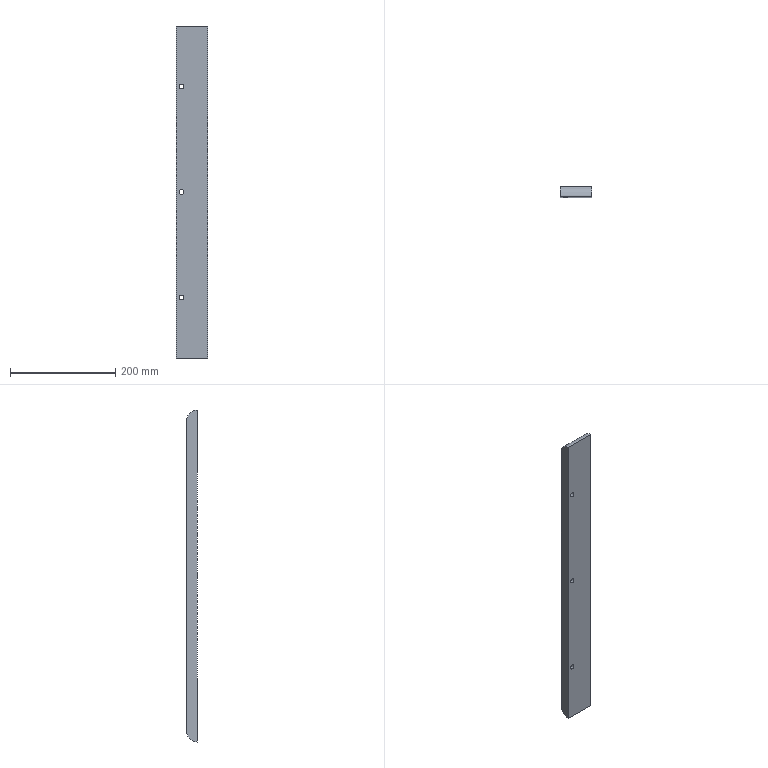Part | 1 solid | 21 faces | box 60 x 20 x 630 mm | volume 738828 mm3 | cylinder 14 | plane 7 | commonest cylinder face diameters 9 x6 15 x6 40 x2
STEP:
#1=CARTESIAN_POINT('',(-20.,1.,-207.5));
#2=VERTEX_POINT('',#1);
#3=CARTESIAN_POINT('',(-20.,1.,-192.5));
#4=VERTEX_POINT('',#3);
#5=CARTESIAN_POINT('',(-20.,1.,-200.));
#6=DIRECTION('',(0.,1.,0.));
#7=DIRECTION('',(0.,0.,1.));
#8=AXIS2_PLACEMENT_3D('',#5,#6,#7);
#9=CIRCLE('',#8,7.5);
#10=EDGE_CURVE('',#2,#4,#9,.T.);
#11=ORIENTED_EDGE('',*,*,#10,.F.);
#12=CARTESIAN_POINT('',(-20.,10.,-207.5));
#13=VERTEX_POINT('',#12);
#14=CARTESIAN_POINT('',(-20.,10.,-207.5));
#15=DIRECTION('',(0.,1.,0.));
#16=VECTOR('',#15,1000.);
#17=LINE('',#14,#16);
#18=EDGE_CURVE('',#2,#13,#17,.T.);
#19=ORIENTED_EDGE('',*,*,#18,.T.);
#20=CARTESIAN_POINT('',(-20.,10.,-192.5));
#21=VERTEX_POINT('',#20);
#22=CARTESIAN_POINT('',(-20.,10.,-200.));
#23=DIRECTION('',(0.,1.,0.));
#24=DIRECTION('',(0.,0.,1.));
#25=AXIS2_PLACEMENT_3D('',#22,#23,#24);
#26=CIRCLE('',#25,7.5);
#27=EDGE_CURVE('',#13,#21,#26,.T.);
#28=ORIENTED_EDGE('',*,*,#27,.T.);
#29=CARTESIAN_POINT('',(-20.,10.,-192.5));
#30=DIRECTION('',(0.,1.,0.));
#31=VECTOR('',#30,1000.);
#32=LINE('',#29,#31);
#33=EDGE_CURVE('',#4,#21,#32,.T.);
#34=ORIENTED_EDGE('',*,*,#33,.F.);
#35=EDGE_LOOP('',(#11,#19,#28,#34));
#36=FACE_OUTER_BOUND('',#35,.T.);
#37=CARTESIAN_POINT('',(-20.,10.,-200.));
#38=DIRECTION('',(0.,1.,0.));
#39=DIRECTION('',(0.,0.,1.));
#40=AXIS2_PLACEMENT_3D('',#37,#38,#39);
#41=CYLINDRICAL_SURFACE('',#40,7.5);
#42=ADVANCED_FACE('',(#36),#41,.F.);
#43=CARTESIAN_POINT('',(-20.,-10.,-204.5));
#44=VERTEX_POINT('',#43);
#45=CARTESIAN_POINT('',(-20.,-10.,-195.5));
#46=VERTEX_POINT('',#45);
#47=CARTESIAN_POINT('',(-20.,-10.,-200.));
#48=DIRECTION('',(0.,1.,0.));
#49=DIRECTION('',(0.,0.,1.));
#50=AXIS2_PLACEMENT_3D('',#47,#48,#49);
#51=CIRCLE('',#50,4.5);
#52=EDGE_CURVE('',#44,#46,#51,.T.);
#53=ORIENTED_EDGE('',*,*,#52,.F.);
#54=CARTESIAN_POINT('',(-20.,1.,-204.5));
#55=VERTEX_POINT('',#54);
#56=CARTESIAN_POINT('',(-20.,10.,-204.5));
#57=DIRECTION('',(0.,1.,0.));
#58=VECTOR('',#57,1000.);
#59=LINE('',#56,#58);
#60=EDGE_CURVE('',#44,#55,#59,.T.);
#61=ORIENTED_EDGE('',*,*,#60,.T.);
#62=CARTESIAN_POINT('',(-20.,1.,-195.5));
#63=VERTEX_POINT('',#62);
#64=CARTESIAN_POINT('',(-20.,1.,-200.));
#65=DIRECTION('',(0.,1.,0.));
#66=DIRECTION('',(0.,0.,1.));
#67=AXIS2_PLACEMENT_3D('',#64,#65,#66);
#68=CIRCLE('',#67,4.5);
#69=EDGE_CURVE('',#55,#63,#68,.T.);
#70=ORIENTED_EDGE('',*,*,#69,.T.);
#71=CARTESIAN_POINT('',(-20.,10.,-195.5));
#72=DIRECTION('',(0.,1.,0.));
#73=VECTOR('',#72,1000.);
#74=LINE('',#71,#73);
#75=EDGE_CURVE('',#46,#63,#74,.T.);
#76=ORIENTED_EDGE('',*,*,#75,.F.);
#77=EDGE_LOOP('',(#53,#61,#70,#76));
#78=FACE_OUTER_BOUND('',#77,.T.);
#79=CARTESIAN_POINT('',(-20.,10.,-200.));
#80=DIRECTION('',(0.,1.,0.));
#81=DIRECTION('',(0.,0.,1.));
#82=AXIS2_PLACEMENT_3D('',#79,#80,#81);
#83=CYLINDRICAL_SURFACE('',#82,4.5);
#84=ADVANCED_FACE('',(#78),#83,.F.);
#85=CARTESIAN_POINT('',(-20.,1.,-7.5));
#86=VERTEX_POINT('',#85);
#87=CARTESIAN_POINT('',(-20.,1.,7.5));
#88=VERTEX_POINT('',#87);
#89=CARTESIAN_POINT('',(-20.,1.,0.));
#90=DIRECTION('',(0.,1.,0.));
#91=DIRECTION('',(0.,0.,1.));
#92=AXIS2_PLACEMENT_3D('',#89,#90,#91);
#93=CIRCLE('',#92,7.5);
#94=EDGE_CURVE('',#86,#88,#93,.T.);
#95=ORIENTED_EDGE('',*,*,#94,.F.);
#96=CARTESIAN_POINT('',(-20.,10.,-7.5));
#97=VERTEX_POINT('',#96);
#98=CARTESIAN_POINT('',(-20.,10.,-7.5));
#99=DIRECTION('',(0.,1.,0.));
#100=VECTOR('',#99,1000.);
#101=LINE('',#98,#100);
#102=EDGE_CURVE('',#86,#97,#101,.T.);
#103=ORIENTED_EDGE('',*,*,#102,.T.);
#104=CARTESIAN_POINT('',(-20.,10.,7.5));
#105=VERTEX_POINT('',#104);
#106=CARTESIAN_POINT('',(-20.,10.,0.));
#107=DIRECTION('',(0.,1.,0.));
#108=DIRECTION('',(0.,0.,1.));
#109=AXIS2_PLACEMENT_3D('',#106,#107,#108);
#110=CIRCLE('',#109,7.5);
#111=EDGE_CURVE('',#97,#105,#110,.T.);
#112=ORIENTED_EDGE('',*,*,#111,.T.);
#113=CARTESIAN_POINT('',(-20.,10.,7.5));
#114=DIRECTION('',(0.,1.,0.));
#115=VECTOR('',#114,1000.);
#116=LINE('',#113,#115);
#117=EDGE_CURVE('',#88,#105,#116,.T.);
#118=ORIENTED_EDGE('',*,*,#117,.F.);
#119=EDGE_LOOP('',(#95,#103,#112,#118));
#120=FACE_OUTER_BOUND('',#119,.T.);
#121=CARTESIAN_POINT('',(-20.,10.,0.));
#122=DIRECTION('',(0.,1.,0.));
#123=DIRECTION('',(0.,0.,1.));
#124=AXIS2_PLACEMENT_3D('',#121,#122,#123);
#125=CYLINDRICAL_SURFACE('',#124,7.5);
#126=ADVANCED_FACE('',(#120),#125,.F.);
#127=CARTESIAN_POINT('',(-20.,-10.,-4.5));
#128=VERTEX_POINT('',#127);
#129=CARTESIAN_POINT('',(-20.,-10.,4.5));
#130=VERTEX_POINT('',#129);
#131=CARTESIAN_POINT('',(-20.,-10.,0.));
#132=DIRECTION('',(0.,1.,0.));
#133=DIRECTION('',(0.,0.,1.));
#134=AXIS2_PLACEMENT_3D('',#131,#132,#133);
#135=CIRCLE('',#134,4.5);
#136=EDGE_CURVE('',#128,#130,#135,.T.);
#137=ORIENTED_EDGE('',*,*,#136,.F.);
#138=CARTESIAN_POINT('',(-20.,1.,-4.5));
#139=VERTEX_POINT('',#138);
#140=CARTESIAN_POINT('',(-20.,10.,-4.5));
#141=DIRECTION('',(0.,1.,0.));
#142=VECTOR('',#141,1000.);
#143=LINE('',#140,#142);
#144=EDGE_CURVE('',#128,#139,#143,.T.);
#145=ORIENTED_EDGE('',*,*,#144,.T.);
#146=CARTESIAN_POINT('',(-20.,1.,4.5));
#147=VERTEX_POINT('',#146);
#148=CARTESIAN_POINT('',(-20.,1.,0.));
#149=DIRECTION('',(0.,1.,0.));
#150=DIRECTION('',(0.,0.,1.));
#151=AXIS2_PLACEMENT_3D('',#148,#149,#150);
#152=CIRCLE('',#151,4.5);
#153=EDGE_CURVE('',#139,#147,#152,.T.);
#154=ORIENTED_EDGE('',*,*,#153,.T.);
#155=CARTESIAN_POINT('',(-20.,10.,4.5));
#156=DIRECTION('',(0.,1.,0.));
#157=VECTOR('',#156,1000.);
#158=LINE('',#155,#157);
#159=EDGE_CURVE('',#130,#147,#158,.T.);
#160=ORIENTED_EDGE('',*,*,#159,.F.);
#161=EDGE_LOOP('',(#137,#145,#154,#160));
#162=FACE_OUTER_BOUND('',#161,.T.);
#163=CARTESIAN_POINT('',(-20.,10.,0.));
#164=DIRECTION('',(0.,1.,0.));
#165=DIRECTION('',(0.,0.,1.));
#166=AXIS2_PLACEMENT_3D('',#163,#164,#165);
#167=CYLINDRICAL_SURFACE('',#166,4.5);
#168=ADVANCED_FACE('',(#162),#167,.F.);
#169=CARTESIAN_POINT('',(-20.,1.,192.5));
#170=VERTEX_POINT('',#169);
#171=CARTESIAN_POINT('',(-20.,1.,207.5));
#172=VERTEX_POINT('',#171);
#173=CARTESIAN_POINT('',(-20.,1.,200.));
#174=DIRECTION('',(0.,1.,0.));
#175=DIRECTION('',(0.,0.,1.));
#176=AXIS2_PLACEMENT_3D('',#173,#174,#175);
#177=CIRCLE('',#176,7.5);
#178=EDGE_CURVE('',#170,#172,#177,.T.);
#179=ORIENTED_EDGE('',*,*,#178,.F.);
#180=CARTESIAN_POINT('',(-20.,10.,192.5));
#181=VERTEX_POINT('',#180);
#182=CARTESIAN_POINT('',(-20.,10.,192.5));
#183=DIRECTION('',(0.,1.,0.));
#184=VECTOR('',#183,1000.);
#185=LINE('',#182,#184);
#186=EDGE_CURVE('',#170,#181,#185,.T.);
#187=ORIENTED_EDGE('',*,*,#186,.T.);
#188=CARTESIAN_POINT('',(-20.,10.,207.5));
#189=VERTEX_POINT('',#188);
#190=CARTESIAN_POINT('',(-20.,10.,200.));
#191=DIRECTION('',(0.,1.,0.));
#192=DIRECTION('',(0.,0.,1.));
#193=AXIS2_PLACEMENT_3D('',#190,#191,#192);
#194=CIRCLE('',#193,7.5);
#195=EDGE_CURVE('',#181,#189,#194,.T.);
#196=ORIENTED_EDGE('',*,*,#195,.T.);
#197=CARTESIAN_POINT('',(-20.,10.,207.5));
#198=DIRECTION('',(0.,1.,0.));
#199=VECTOR('',#198,1000.);
#200=LINE('',#197,#199);
#201=EDGE_CURVE('',#172,#189,#200,.T.);
#202=ORIENTED_EDGE('',*,*,#201,.F.);
#203=EDGE_LOOP('',(#179,#187,#196,#202));
#204=FACE_OUTER_BOUND('',#203,.T.);
#205=CARTESIAN_POINT('',(-20.,10.,200.));
#206=DIRECTION('',(0.,1.,0.));
#207=DIRECTION('',(0.,0.,1.));
#208=AXIS2_PLACEMENT_3D('',#205,#206,#207);
#209=CYLINDRICAL_SURFACE('',#208,7.5);
#210=ADVANCED_FACE('',(#204),#209,.F.);
#211=CARTESIAN_POINT('',(-20.,-10.,195.5));
#212=VERTEX_POINT('',#211);
#213=CARTESIAN_POINT('',(-20.,-10.,204.5));
#214=VERTEX_POINT('',#213);
#215=CARTESIAN_POINT('',(-20.,-10.,200.));
#216=DIRECTION('',(0.,1.,0.));
#217=DIRECTION('',(0.,0.,1.));
#218=AXIS2_PLACEMENT_3D('',#215,#216,#217);
#219=CIRCLE('',#218,4.5);
#220=EDGE_CURVE('',#212,#214,#219,.T.);
#221=ORIENTED_EDGE('',*,*,#220,.F.);
#222=CARTESIAN_POINT('',(-20.,1.,195.5));
#223=VERTEX_POINT('',#222);
#224=CARTESIAN_POINT('',(-20.,10.,195.5));
#225=DIRECTION('',(0.,1.,0.));
#226=VECTOR('',#225,1000.);
#227=LINE('',#224,#226);
#228=EDGE_CURVE('',#212,#223,#227,.T.);
#229=ORIENTED_EDGE('',*,*,#228,.T.);
#230=CARTESIAN_POINT('',(-20.,1.,204.5));
#231=VERTEX_POINT('',#230);
#232=CARTESIAN_POINT('',(-20.,1.,200.));
#233=DIRECTION('',(0.,1.,0.));
#234=DIRECTION('',(0.,0.,1.));
#235=AXIS2_PLACEMENT_3D('',#232,#233,#234);
#236=CIRCLE('',#235,4.5);
#237=EDGE_CURVE('',#223,#231,#236,.T.);
#238=ORIENTED_EDGE('',*,*,#237,.T.);
#239=CARTESIAN_POINT('',(-20.,10.,204.5));
#240=DIRECTION('',(0.,1.,0.));
#241=VECTOR('',#240,1000.);
#242=LINE('',#239,#241);
#243=EDGE_CURVE('',#214,#231,#242,.T.);
#244=ORIENTED_EDGE('',*,*,#243,.F.);
#245=EDGE_LOOP('',(#221,#229,#238,#244));
#246=FACE_OUTER_BOUND('',#245,.T.);
#247=CARTESIAN_POINT('',(-20.,10.,200.));
#248=DIRECTION('',(0.,1.,0.));
#249=DIRECTION('',(0.,0.,1.));
#250=AXIS2_PLACEMENT_3D('',#247,#248,#249);
#251=CYLINDRICAL_SURFACE('',#250,4.5);
#252=ADVANCED_FACE('',(#246),#251,.F.);
#253=CARTESIAN_POINT('',(30.,10.,295.));
#254=VERTEX_POINT('',#253);
#255=CARTESIAN_POINT('',(30.,10.,-295.));
#256=VERTEX_POINT('',#255);
#257=CARTESIAN_POINT('',(30.,10.,315.));
#258=DIRECTION('',(0.,0.,-1.));
#259=VECTOR('',#258,1000.);
#260=LINE('',#257,#259);
#261=EDGE_CURVE('',#254,#256,#260,.T.);
#262=ORIENTED_EDGE('',*,*,#261,.F.);
#263=CARTESIAN_POINT('',(30.,-10.,315.));
#264=VERTEX_POINT('',#263);
#265=CARTESIAN_POINT('',(30.,-10.,295.));
#266=DIRECTION('',(1.,0.,0.));
#267=DIRECTION('',(0.,-1.,0.));
#268=AXIS2_PLACEMENT_3D('',#265,#266,#267);
#269=CIRCLE('',#268,20.);
#270=EDGE_CURVE('',#254,#264,#269,.T.);
#271=ORIENTED_EDGE('',*,*,#270,.T.);
#272=CARTESIAN_POINT('',(30.,-10.,-315.));
#273=VERTEX_POINT('',#272);
#274=CARTESIAN_POINT('',(30.,-10.,315.));
#275=DIRECTION('',(0.,0.,-1.));
#276=VECTOR('',#275,1000.);
#277=LINE('',#274,#276);
#278=EDGE_CURVE('',#264,#273,#277,.T.);
#279=ORIENTED_EDGE('',*,*,#278,.T.);
#280=CARTESIAN_POINT('',(30.,-10.,-295.));
#281=DIRECTION('',(1.,0.,0.));
#282=DIRECTION('',(0.,-1.,0.));
#283=AXIS2_PLACEMENT_3D('',#280,#281,#282);
#284=CIRCLE('',#283,20.);
#285=EDGE_CURVE('',#273,#256,#284,.T.);
#286=ORIENTED_EDGE('',*,*,#285,.T.);
#287=EDGE_LOOP('',(#262,#271,#279,#286));
#288=FACE_OUTER_BOUND('',#287,.T.);
#289=CARTESIAN_POINT('',(30.,10.,315.));
#290=DIRECTION('',(-1.,0.,0.));
#291=DIRECTION('',(0.,-1.,0.));
#292=AXIS2_PLACEMENT_3D('',#289,#290,#291);
#293=PLANE('',#292);
#294=ADVANCED_FACE('',(#288),#293,.F.);
#295=CARTESIAN_POINT('',(-20.,10.,-200.));
#296=DIRECTION('',(0.,1.,0.));
#297=DIRECTION('',(0.,0.,1.));
#298=AXIS2_PLACEMENT_3D('',#295,#296,#297);
#299=CIRCLE('',#298,7.5);
#300=EDGE_CURVE('',#21,#13,#299,.T.);
#301=ORIENTED_EDGE('',*,*,#300,.F.);
#302=ORIENTED_EDGE('',*,*,#27,.F.);
#303=EDGE_LOOP('',(#301,#302));
#304=FACE_BOUND('',#303,.T.);
#305=CARTESIAN_POINT('',(-20.,10.,0.));
#306=DIRECTION('',(0.,1.,0.));
#307=DIRECTION('',(0.,0.,1.));
#308=AXIS2_PLACEMENT_3D('',#305,#306,#307);
#309=CIRCLE('',#308,7.5);
#310=EDGE_CURVE('',#105,#97,#309,.T.);
#311=ORIENTED_EDGE('',*,*,#310,.F.);
#312=ORIENTED_EDGE('',*,*,#111,.F.);
#313=EDGE_LOOP('',(#311,#312));
#314=FACE_BOUND('',#313,.T.);
#315=CARTESIAN_POINT('',(-20.,10.,200.));
#316=DIRECTION('',(0.,1.,0.));
#317=DIRECTION('',(0.,0.,1.));
#318=AXIS2_PLACEMENT_3D('',#315,#316,#317);
#319=CIRCLE('',#318,7.5);
#320=EDGE_CURVE('',#189,#181,#319,.T.);
#321=ORIENTED_EDGE('',*,*,#320,.F.);
#322=ORIENTED_EDGE('',*,*,#195,.F.);
#323=EDGE_LOOP('',(#321,#322));
#324=FACE_BOUND('',#323,.T.);
#325=CARTESIAN_POINT('',(-30.,10.,295.));
#326=VERTEX_POINT('',#325);
#327=CARTESIAN_POINT('',(-30.,10.,-295.));
#328=VERTEX_POINT('',#327);
#329=CARTESIAN_POINT('',(-30.,10.,315.));
#330=DIRECTION('',(0.,0.,-1.));
#331=VECTOR('',#330,1000.);
#332=LINE('',#329,#331);
#333=EDGE_CURVE('',#326,#328,#332,.T.);
#334=ORIENTED_EDGE('',*,*,#333,.F.);
#335=CARTESIAN_POINT('',(30.,10.,295.));
#336=DIRECTION('',(1.,0.,0.));
#337=VECTOR('',#336,1000.);
#338=LINE('',#335,#337);
#339=EDGE_CURVE('',#326,#254,#338,.T.);
#340=ORIENTED_EDGE('',*,*,#339,.T.);
#341=ORIENTED_EDGE('',*,*,#261,.T.);
#342=CARTESIAN_POINT('',(-30.,10.,-295.));
#343=DIRECTION('',(-1.,0.,0.));
#344=VECTOR('',#343,1000.);
#345=LINE('',#342,#344);
#346=EDGE_CURVE('',#256,#328,#345,.T.);
#347=ORIENTED_EDGE('',*,*,#346,.T.);
#348=EDGE_LOOP('',(#334,#340,#341,#347));
#349=FACE_OUTER_BOUND('',#348,.T.);
#350=CARTESIAN_POINT('',(-30.,10.,315.));
#351=DIRECTION('',(0.,-1.,0.));
#352=DIRECTION('',(0.,0.,-1.));
#353=AXIS2_PLACEMENT_3D('',#350,#351,#352);
#354=PLANE('',#353);
#355=ADVANCED_FACE('',(#304,#314,#324,#349),#354,.F.);
#356=CARTESIAN_POINT('',(-30.,-10.,315.));
#357=VERTEX_POINT('',#356);
#358=CARTESIAN_POINT('',(-30.,-10.,-315.));
#359=VERTEX_POINT('',#358);
#360=CARTESIAN_POINT('',(-30.,-10.,315.));
#361=DIRECTION('',(0.,0.,-1.));
#362=VECTOR('',#361,1000.);
#363=LINE('',#360,#362);
#364=EDGE_CURVE('',#357,#359,#363,.T.);
#365=ORIENTED_EDGE('',*,*,#364,.F.);
#366=CARTESIAN_POINT('',(-30.,-10.,295.));
#367=DIRECTION('',(-1.,0.,0.));
#368=DIRECTION('',(0.,1.,0.));
#369=AXIS2_PLACEMENT_3D('',#366,#367,#368);
#370=CIRCLE('',#369,20.);
#371=EDGE_CURVE('',#357,#326,#370,.T.);
#372=ORIENTED_EDGE('',*,*,#371,.T.);
#373=ORIENTED_EDGE('',*,*,#333,.T.);
#374=CARTESIAN_POINT('',(-30.,-10.,-295.));
#375=DIRECTION('',(-1.,0.,0.));
#376=DIRECTION('',(0.,1.,0.));
#377=AXIS2_PLACEMENT_3D('',#374,#375,#376);
#378=CIRCLE('',#377,20.);
#379=EDGE_CURVE('',#328,#359,#378,.T.);
#380=ORIENTED_EDGE('',*,*,#379,.T.);
#381=EDGE_LOOP('',(#365,#372,#373,#380));
#382=FACE_OUTER_BOUND('',#381,.T.);
#383=CARTESIAN_POINT('',(-30.,10.,315.));
#384=DIRECTION('',(1.,0.,0.));
#385=DIRECTION('',(0.,1.,0.));
#386=AXIS2_PLACEMENT_3D('',#383,#384,#385);
#387=PLANE('',#386);
#388=ADVANCED_FACE('',(#382),#387,.F.);
#389=CARTESIAN_POINT('',(-20.,-10.,-200.));
#390=DIRECTION('',(0.,1.,0.));
#391=DIRECTION('',(0.,0.,1.));
#392=AXIS2_PLACEMENT_3D('',#389,#390,#391);
#393=CIRCLE('',#392,4.5);
#394=EDGE_CURVE('',#46,#44,#393,.T.);
#395=ORIENTED_EDGE('',*,*,#394,.T.);
#396=ORIENTED_EDGE('',*,*,#52,.T.);
#397=EDGE_LOOP('',(#395,#396));
#398=FACE_BOUND('',#397,.T.);
#399=CARTESIAN_POINT('',(-20.,-10.,0.));
#400=DIRECTION('',(0.,1.,0.));
#401=DIRECTION('',(0.,0.,1.));
#402=AXIS2_PLACEMENT_3D('',#399,#400,#401);
#403=CIRCLE('',#402,4.5);
#404=EDGE_CURVE('',#130,#128,#403,.T.);
#405=ORIENTED_EDGE('',*,*,#404,.T.);
#406=ORIENTED_EDGE('',*,*,#136,.T.);
#407=EDGE_LOOP('',(#405,#406));
#408=FACE_BOUND('',#407,.T.);
#409=CARTESIAN_POINT('',(-20.,-10.,200.));
#410=DIRECTION('',(0.,1.,0.));
#411=DIRECTION('',(0.,0.,1.));
#412=AXIS2_PLACEMENT_3D('',#409,#410,#411);
#413=CIRCLE('',#412,4.5);
#414=EDGE_CURVE('',#214,#212,#413,.T.);
#415=ORIENTED_EDGE('',*,*,#414,.T.);
#416=ORIENTED_EDGE('',*,*,#220,.T.);
#417=EDGE_LOOP('',(#415,#416));
#418=FACE_BOUND('',#417,.T.);
#419=CARTESIAN_POINT('',(-30.,-10.,-315.));
#420=DIRECTION('',(1.,0.,0.));
#421=VECTOR('',#420,1000.);
#422=LINE('',#419,#421);
#423=EDGE_CURVE('',#359,#273,#422,.T.);
#424=ORIENTED_EDGE('',*,*,#423,.T.);
#425=ORIENTED_EDGE('',*,*,#278,.F.);
#426=CARTESIAN_POINT('',(-30.,-10.,315.));
#427=DIRECTION('',(1.,0.,0.));
#428=VECTOR('',#427,1000.);
#429=LINE('',#426,#428);
#430=EDGE_CURVE('',#357,#264,#429,.T.);
#431=ORIENTED_EDGE('',*,*,#430,.F.);
#432=ORIENTED_EDGE('',*,*,#364,.T.);
#433=EDGE_LOOP('',(#424,#425,#431,#432));
#434=FACE_OUTER_BOUND('',#433,.T.);
#435=CARTESIAN_POINT('',(-30.,-10.,315.));
#436=DIRECTION('',(0.,1.,0.));
#437=DIRECTION('',(0.,0.,1.));
#438=AXIS2_PLACEMENT_3D('',#435,#436,#437);
#439=PLANE('',#438);
#440=ADVANCED_FACE('',(#398,#408,#418,#434),#439,.F.);
#441=ORIENTED_EDGE('',*,*,#228,.F.);
#442=ORIENTED_EDGE('',*,*,#414,.F.);
#443=ORIENTED_EDGE('',*,*,#243,.T.);
#444=CARTESIAN_POINT('',(-20.,1.,200.));
#445=DIRECTION('',(0.,1.,0.));
#446=DIRECTION('',(0.,0.,1.));
#447=AXIS2_PLACEMENT_3D('',#444,#445,#446);
#448=CIRCLE('',#447,4.5);
#449=EDGE_CURVE('',#231,#223,#448,.T.);
#450=ORIENTED_EDGE('',*,*,#449,.T.);
#451=EDGE_LOOP('',(#441,#442,#443,#450));
#452=FACE_OUTER_BOUND('',#451,.T.);
#453=CARTESIAN_POINT('',(-20.,10.,200.));
#454=DIRECTION('',(0.,1.,0.));
#455=DIRECTION('',(0.,0.,1.));
#456=AXIS2_PLACEMENT_3D('',#453,#454,#455);
#457=CYLINDRICAL_SURFACE('',#456,4.5);
#458=ADVANCED_FACE('',(#452),#457,.F.);
#459=ORIENTED_EDGE('',*,*,#449,.F.);
#460=ORIENTED_EDGE('',*,*,#237,.F.);
#461=EDGE_LOOP('',(#459,#460));
#462=FACE_BOUND('',#461,.T.);
#463=CARTESIAN_POINT('',(-20.,1.,200.));
#464=DIRECTION('',(0.,1.,0.));
#465=DIRECTION('',(0.,0.,1.));
#466=AXIS2_PLACEMENT_3D('',#463,#464,#465);
#467=CIRCLE('',#466,7.5);
#468=EDGE_CURVE('',#172,#170,#467,.T.);
#469=ORIENTED_EDGE('',*,*,#468,.T.);
#470=ORIENTED_EDGE('',*,*,#178,.T.);
#471=EDGE_LOOP('',(#469,#470));
#472=FACE_OUTER_BOUND('',#471,.T.);
#473=CARTESIAN_POINT('',(-15.5,1.,200.));
#474=DIRECTION('',(0.,-1.,0.));
#475=DIRECTION('',(0.,0.,-1.));
#476=AXIS2_PLACEMENT_3D('',#473,#474,#475);
#477=PLANE('',#476);
#478=ADVANCED_FACE('',(#462,#472),#477,.F.);
#479=ORIENTED_EDGE('',*,*,#186,.F.);
#480=ORIENTED_EDGE('',*,*,#468,.F.);
#481=ORIENTED_EDGE('',*,*,#201,.T.);
#482=ORIENTED_EDGE('',*,*,#320,.T.);
#483=EDGE_LOOP('',(#479,#480,#481,#482));
#484=FACE_OUTER_BOUND('',#483,.T.);
#485=CARTESIAN_POINT('',(-20.,10.,200.));
#486=DIRECTION('',(0.,1.,0.));
#487=DIRECTION('',(0.,0.,1.));
#488=AXIS2_PLACEMENT_3D('',#485,#486,#487);
#489=CYLINDRICAL_SURFACE('',#488,7.5);
#490=ADVANCED_FACE('',(#484),#489,.F.);
#491=ORIENTED_EDGE('',*,*,#144,.F.);
#492=ORIENTED_EDGE('',*,*,#404,.F.);
#493=ORIENTED_EDGE('',*,*,#159,.T.);
#494=CARTESIAN_POINT('',(-20.,1.,0.));
#495=DIRECTION('',(0.,1.,0.));
#496=DIRECTION('',(0.,0.,1.));
#497=AXIS2_PLACEMENT_3D('',#494,#495,#496);
#498=CIRCLE('',#497,4.5);
#499=EDGE_CURVE('',#147,#139,#498,.T.);
#500=ORIENTED_EDGE('',*,*,#499,.T.);
#501=EDGE_LOOP('',(#491,#492,#493,#500));
#502=FACE_OUTER_BOUND('',#501,.T.);
#503=CARTESIAN_POINT('',(-20.,10.,0.));
#504=DIRECTION('',(0.,1.,0.));
#505=DIRECTION('',(0.,0.,1.));
#506=AXIS2_PLACEMENT_3D('',#503,#504,#505);
#507=CYLINDRICAL_SURFACE('',#506,4.5);
#508=ADVANCED_FACE('',(#502),#507,.F.);
#509=ORIENTED_EDGE('',*,*,#499,.F.);
#510=ORIENTED_EDGE('',*,*,#153,.F.);
#511=EDGE_LOOP('',(#509,#510));
#512=FACE_BOUND('',#511,.T.);
#513=CARTESIAN_POINT('',(-20.,1.,0.));
#514=DIRECTION('',(0.,1.,0.));
#515=DIRECTION('',(0.,0.,1.));
#516=AXIS2_PLACEMENT_3D('',#513,#514,#515);
#517=CIRCLE('',#516,7.5);
#518=EDGE_CURVE('',#88,#86,#517,.T.);
#519=ORIENTED_EDGE('',*,*,#518,.T.);
#520=ORIENTED_EDGE('',*,*,#94,.T.);
#521=EDGE_LOOP('',(#519,#520));
#522=FACE_OUTER_BOUND('',#521,.T.);
#523=CARTESIAN_POINT('',(-15.5,1.,0.));
#524=DIRECTION('',(0.,-1.,0.));
#525=DIRECTION('',(0.,0.,-1.));
#526=AXIS2_PLACEMENT_3D('',#523,#524,#525);
#527=PLANE('',#526);
#528=ADVANCED_FACE('',(#512,#522),#527,.F.);
#529=ORIENTED_EDGE('',*,*,#102,.F.);
#530=ORIENTED_EDGE('',*,*,#518,.F.);
#531=ORIENTED_EDGE('',*,*,#117,.T.);
#532=ORIENTED_EDGE('',*,*,#310,.T.);
#533=EDGE_LOOP('',(#529,#530,#531,#532));
#534=FACE_OUTER_BOUND('',#533,.T.);
#535=CARTESIAN_POINT('',(-20.,10.,0.));
#536=DIRECTION('',(0.,1.,0.));
#537=DIRECTION('',(0.,0.,1.));
#538=AXIS2_PLACEMENT_3D('',#535,#536,#537);
#539=CYLINDRICAL_SURFACE('',#538,7.5);
#540=ADVANCED_FACE('',(#534),#539,.F.);
#541=ORIENTED_EDGE('',*,*,#60,.F.);
#542=ORIENTED_EDGE('',*,*,#394,.F.);
#543=ORIENTED_EDGE('',*,*,#75,.T.);
#544=CARTESIAN_POINT('',(-20.,1.,-200.));
#545=DIRECTION('',(0.,1.,0.));
#546=DIRECTION('',(0.,0.,1.));
#547=AXIS2_PLACEMENT_3D('',#544,#545,#546);
#548=CIRCLE('',#547,4.5);
#549=EDGE_CURVE('',#63,#55,#548,.T.);
#550=ORIENTED_EDGE('',*,*,#549,.T.);
#551=EDGE_LOOP('',(#541,#542,#543,#550));
#552=FACE_OUTER_BOUND('',#551,.T.);
#553=CARTESIAN_POINT('',(-20.,10.,-200.));
#554=DIRECTION('',(0.,1.,0.));
#555=DIRECTION('',(0.,0.,1.));
#556=AXIS2_PLACEMENT_3D('',#553,#554,#555);
#557=CYLINDRICAL_SURFACE('',#556,4.5);
#558=ADVANCED_FACE('',(#552),#557,.F.);
#559=ORIENTED_EDGE('',*,*,#549,.F.);
#560=ORIENTED_EDGE('',*,*,#69,.F.);
#561=EDGE_LOOP('',(#559,#560));
#562=FACE_BOUND('',#561,.T.);
#563=CARTESIAN_POINT('',(-20.,1.,-200.));
#564=DIRECTION('',(0.,1.,0.));
#565=DIRECTION('',(0.,0.,1.));
#566=AXIS2_PLACEMENT_3D('',#563,#564,#565);
#567=CIRCLE('',#566,7.5);
#568=EDGE_CURVE('',#4,#2,#567,.T.);
#569=ORIENTED_EDGE('',*,*,#568,.T.);
#570=ORIENTED_EDGE('',*,*,#10,.T.);
#571=EDGE_LOOP('',(#569,#570));
#572=FACE_OUTER_BOUND('',#571,.T.);
#573=CARTESIAN_POINT('',(-15.5,1.,-200.));
#574=DIRECTION('',(0.,-1.,0.));
#575=DIRECTION('',(0.,0.,-1.));
#576=AXIS2_PLACEMENT_3D('',#573,#574,#575);
#577=PLANE('',#576);
#578=ADVANCED_FACE('',(#562,#572),#577,.F.);
#579=ORIENTED_EDGE('',*,*,#18,.F.);
#580=ORIENTED_EDGE('',*,*,#568,.F.);
#581=ORIENTED_EDGE('',*,*,#33,.T.);
#582=ORIENTED_EDGE('',*,*,#300,.T.);
#583=EDGE_LOOP('',(#579,#580,#581,#582));
#584=FACE_OUTER_BOUND('',#583,.T.);
#585=CARTESIAN_POINT('',(-20.,10.,-200.));
#586=DIRECTION('',(0.,1.,0.));
#587=DIRECTION('',(0.,0.,1.));
#588=AXIS2_PLACEMENT_3D('',#585,#586,#587);
#589=CYLINDRICAL_SURFACE('',#588,7.5);
#590=ADVANCED_FACE('',(#584),#589,.F.);
#591=ORIENTED_EDGE('',*,*,#270,.F.);
#592=ORIENTED_EDGE('',*,*,#339,.F.);
#593=ORIENTED_EDGE('',*,*,#371,.F.);
#594=ORIENTED_EDGE('',*,*,#430,.T.);
#595=EDGE_LOOP('',(#591,#592,#593,#594));
#596=FACE_OUTER_BOUND('',#595,.T.);
#597=CARTESIAN_POINT('',(0.,-10.,295.));
#598=DIRECTION('',(1.,0.,0.));
#599=DIRECTION('',(0.,0.,-1.));
#600=AXIS2_PLACEMENT_3D('',#597,#598,#599);
#601=CYLINDRICAL_SURFACE('',#600,20.);
#602=ADVANCED_FACE('',(#596),#601,.T.);
#603=ORIENTED_EDGE('',*,*,#285,.F.);
#604=ORIENTED_EDGE('',*,*,#423,.F.);
#605=ORIENTED_EDGE('',*,*,#379,.F.);
#606=ORIENTED_EDGE('',*,*,#346,.F.);
#607=EDGE_LOOP('',(#603,#604,#605,#606));
#608=FACE_OUTER_BOUND('',#607,.T.);
#609=CARTESIAN_POINT('',(-30.,-10.,-295.));
#610=DIRECTION('',(-1.,0.,0.));
#611=DIRECTION('',(0.,0.,1.));
#612=AXIS2_PLACEMENT_3D('',#609,#610,#611);
#613=CYLINDRICAL_SURFACE('',#612,20.);
#614=ADVANCED_FACE('',(#608),#613,.T.);
#615=CLOSED_SHELL('',(#42,#84,#126,#168,#210,#252,#294,#355,#388,#440,#458,#478,#490,#508,#528,#540,#558,#578,#590,#602,#614));
#616=MANIFOLD_SOLID_BREP('',#615);
#617=CARTESIAN_POINT('',(0.,0.,0.));
#618=DIRECTION('',(0.,0.,1.));
#619=DIRECTION('',(1.,0.,0.));
#620=AXIS2_PLACEMENT_3D('',#617,#618,#619);
#621=(LENGTH_UNIT()NAMED_UNIT(*)SI_UNIT(.MILLI.,.METRE.));
#622=UNCERTAINTY_MEASURE_WITH_UNIT(LENGTH_MEASURE(0.00001),#621,'','');
#623=(NAMED_UNIT(*)PLANE_ANGLE_UNIT()SI_UNIT($,.RADIAN.));
#624=(NAMED_UNIT(*)SI_UNIT($,.STERADIAN.)SOLID_ANGLE_UNIT());
#625=(GEOMETRIC_REPRESENTATION_CONTEXT(3)GLOBAL_UNCERTAINTY_ASSIGNED_CONTEXT((#622))GLOBAL_UNIT_ASSIGNED_CONTEXT((#621,#623,#624))REPRESENTATION_CONTEXT('',''));
#626=ADVANCED_BREP_SHAPE_REPRESENTATION('',(#616,#620),#625);